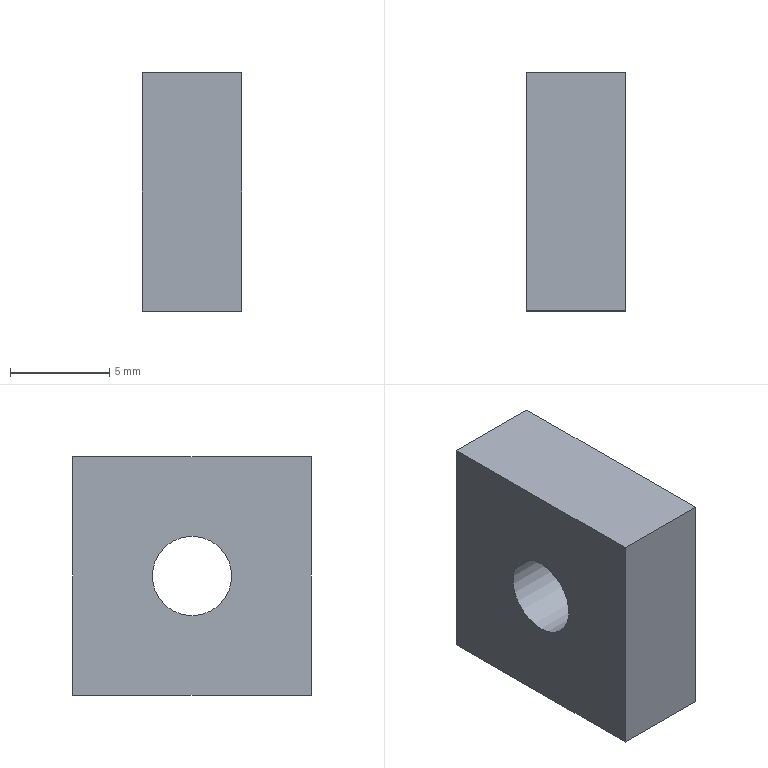Part | STEP file | solid 125 | 1 solid | 7 faces | box 5 x 12 x 12 mm | volume 657.168 mm3 | plane 6 | cylinder 1 | commonest cylinder face diameters 4 x1